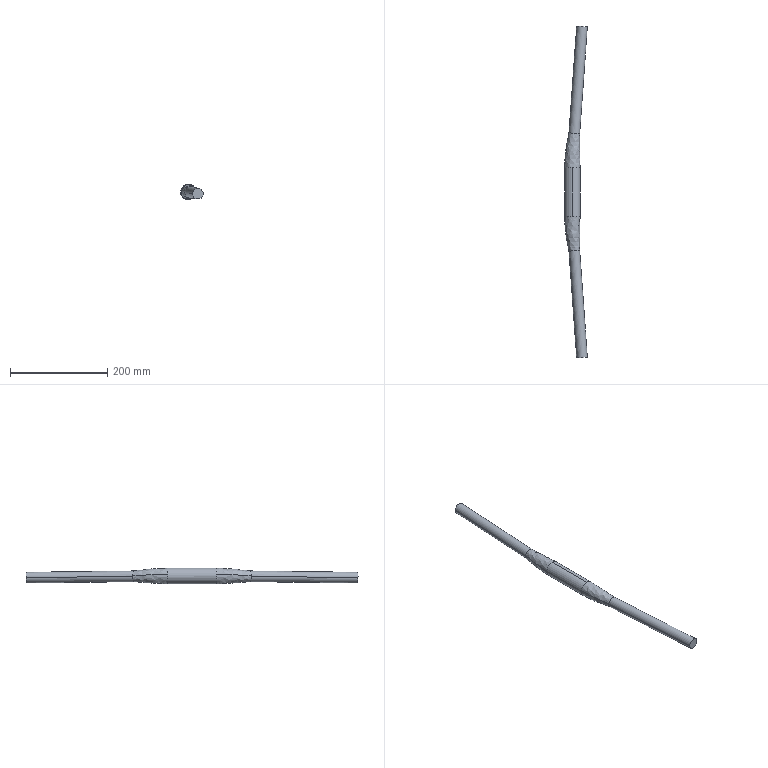Part | SolidWorks | features BaseBody 1 | 1 solid | 12 faces | box 46.593 x 681.596 x 31.8 mm | volume 335473 mm3 | cylinder 6 | spline 4 | plane 2 | commonest cylinder face diameters 22 x4 31.8 x2